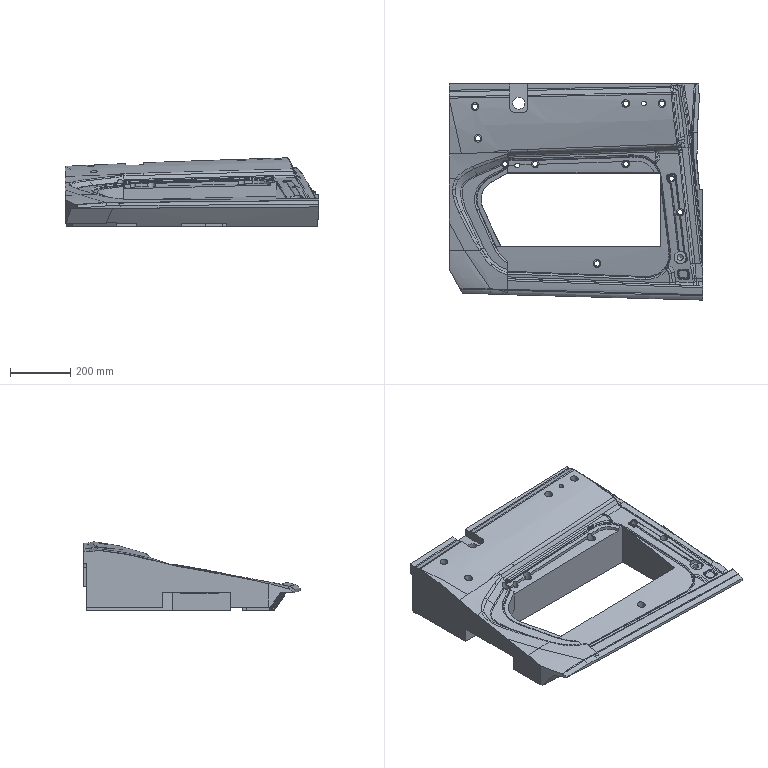Part | NX | features solid 2 | 1 solid | 586 faces | box 843.903 x 716.261 x 226.408 mm | volume 38412472 mm3 | spline 456 | plane 102 | cylinder 27 | cone 1 | commonest cylinder face diameters 25.5 x9 17 x5 17.5 x4 16 x3 20 x2 30 x2